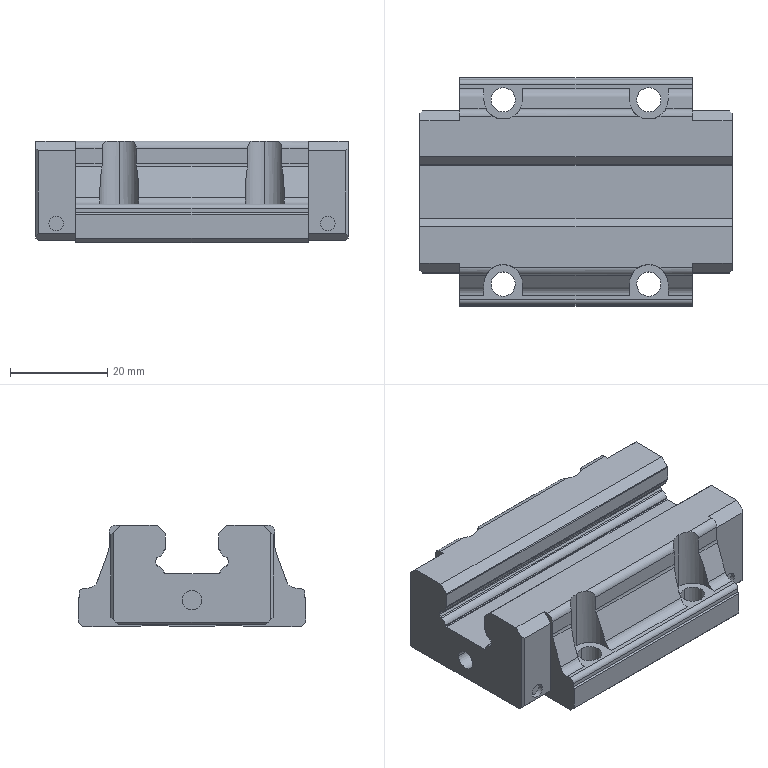Part | STEP file | SHS15C block-Part-1 | 1 solid | 149 faces | box 64.4 x 47 x 21 mm | volume 41708 mm3 | plane 84 | cylinder 65 | commonest cylinder face diameters 4 x16 3 x14 0.6 x8 5 x8 8 x6 2.861 x4